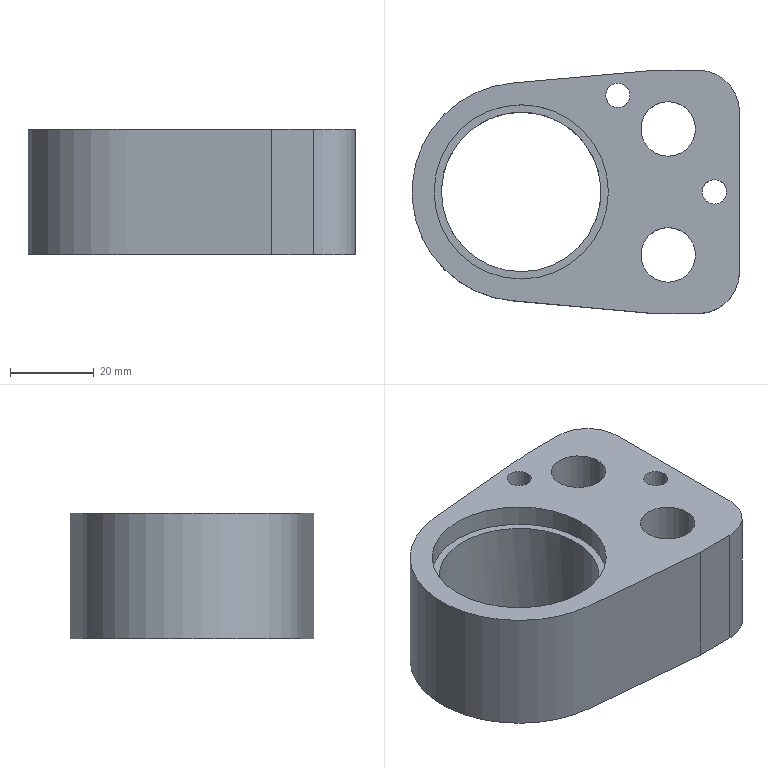Part | NX | features solid 2 | 1 solid | 27 faces | box 78 x 58 x 30 mm | volume 68434 mm3 | plane 14 | cylinder 13 | commonest cylinder face diameters 5.8 x2 8 x2 13 x2 19 x2 20 x2 38 x1
STEP:
#1=CARTESIAN_POINT('',(-809.43,-188.249,101.));
#2=VERTEX_POINT('',#1);
#3=CARTESIAN_POINT('',(-809.43,-188.249,131.));
#4=VERTEX_POINT('',#3);
#5=CARTESIAN_POINT('',(-809.43,-188.249,101.));
#6=DIRECTION('',(0.,0.,1.));
#7=VECTOR('',#6,1000.);
#8=LINE('',#5,#7);
#9=EDGE_CURVE('',#2,#4,#8,.T.);
#10=ORIENTED_EDGE('',*,*,#9,.F.);
#11=CARTESIAN_POINT('',(-809.43,-188.249,101.));
#12=VERTEX_POINT('',#11);
#13=CARTESIAN_POINT('',(-809.43,-214.144,101.));
#14=DIRECTION('',(0.,-1.,0.));
#15=VECTOR('',#14,1000.);
#16=LINE('',#13,#15);
#17=EDGE_CURVE('',#2,#12,#16,.T.);
#18=ORIENTED_EDGE('',*,*,#17,.T.);
#19=CARTESIAN_POINT('',(-809.43,-188.249,131.));
#20=VERTEX_POINT('',#19);
#21=CARTESIAN_POINT('',(-809.43,-188.249,131.));
#22=DIRECTION('',(0.,0.,-1.));
#23=VECTOR('',#22,1000.);
#24=LINE('',#21,#23);
#25=EDGE_CURVE('',#20,#12,#24,.T.);
#26=ORIENTED_EDGE('',*,*,#25,.F.);
#27=CARTESIAN_POINT('',(-809.43,-214.144,131.));
#28=DIRECTION('',(0.,1.,0.));
#29=VECTOR('',#28,1000.);
#30=LINE('',#27,#29);
#31=EDGE_CURVE('',#20,#4,#30,.T.);
#32=ORIENTED_EDGE('',*,*,#31,.T.);
#33=EDGE_LOOP('',(#10,#18,#26,#32));
#34=FACE_BOUND('',#33,.T.);
#35=CARTESIAN_POINT('',(-809.43,-214.144,101.));
#36=DIRECTION('',(-1.,0.,0.));
#37=DIRECTION('',(0.,0.,1.));
#38=AXIS2_PLACEMENT_3D('',#35,#36,#37);
#39=PLANE('',#38);
#40=ADVANCED_FACE('',(#34),#39,.T.);
#41=CARTESIAN_POINT('',(-775.09,-185.144,131.));
#42=VERTEX_POINT('',#41);
#43=CARTESIAN_POINT('',(-795.009,-186.945,131.));
#44=DIRECTION('',(-0.9959,-0.09007,0.));
#45=VECTOR('',#44,1000.);
#46=LINE('',#43,#45);
#47=EDGE_CURVE('',#42,#4,#46,.T.);
#48=ORIENTED_EDGE('',*,*,#47,.T.);
#49=ORIENTED_EDGE('',*,*,#31,.F.);
#50=CARTESIAN_POINT('',(-809.43,-240.038,131.));
#51=VERTEX_POINT('',#50);
#52=CARTESIAN_POINT('',(-807.09,-214.144,131.));
#53=DIRECTION('',(0.,0.,-1.));
#54=DIRECTION('',(0.,-1.,0.));
#55=AXIS2_PLACEMENT_3D('',#52,#53,#54);
#56=CIRCLE('',#55,26.);
#57=EDGE_CURVE('',#51,#20,#56,.T.);
#58=ORIENTED_EDGE('',*,*,#57,.F.);
#59=CARTESIAN_POINT('',(-809.43,-240.038,131.));
#60=VERTEX_POINT('',#59);
#61=CARTESIAN_POINT('',(-809.43,-214.144,131.));
#62=DIRECTION('',(0.,1.,0.));
#63=VECTOR('',#62,1000.);
#64=LINE('',#61,#63);
#65=EDGE_CURVE('',#60,#51,#64,.T.);
#66=ORIENTED_EDGE('',*,*,#65,.F.);
#67=CARTESIAN_POINT('',(-775.09,-243.144,131.));
#68=VERTEX_POINT('',#67);
#69=CARTESIAN_POINT('',(-795.009,-241.342,131.));
#70=DIRECTION('',(0.9959,-0.09007,0.));
#71=VECTOR('',#70,1000.);
#72=LINE('',#69,#71);
#73=EDGE_CURVE('',#60,#68,#72,.T.);
#74=ORIENTED_EDGE('',*,*,#73,.T.);
#75=CARTESIAN_POINT('',(-765.09,-243.144,131.));
#76=VERTEX_POINT('',#75);
#77=CARTESIAN_POINT('',(-792.26,-243.144,131.));
#78=DIRECTION('',(-1.,0.,0.));
#79=VECTOR('',#78,1000.);
#80=LINE('',#77,#79);
#81=EDGE_CURVE('',#76,#68,#80,.T.);
#82=ORIENTED_EDGE('',*,*,#81,.F.);
#83=CARTESIAN_POINT('',(-755.09,-233.144,131.));
#84=VERTEX_POINT('',#83);
#85=CARTESIAN_POINT('',(-765.09,-233.144,131.));
#86=DIRECTION('',(0.,0.,1.));
#87=DIRECTION('',(0.,1.,0.));
#88=AXIS2_PLACEMENT_3D('',#85,#86,#87);
#89=CIRCLE('',#88,10.);
#90=EDGE_CURVE('',#76,#84,#89,.T.);
#91=ORIENTED_EDGE('',*,*,#90,.T.);
#92=CARTESIAN_POINT('',(-755.09,-195.144,131.));
#93=VERTEX_POINT('',#92);
#94=CARTESIAN_POINT('',(-755.09,-214.144,131.));
#95=DIRECTION('',(0.,-1.,0.));
#96=VECTOR('',#95,1000.);
#97=LINE('',#94,#96);
#98=EDGE_CURVE('',#93,#84,#97,.T.);
#99=ORIENTED_EDGE('',*,*,#98,.F.);
#100=CARTESIAN_POINT('',(-765.09,-185.144,131.));
#101=VERTEX_POINT('',#100);
#102=CARTESIAN_POINT('',(-765.09,-195.144,131.));
#103=DIRECTION('',(0.,0.,1.));
#104=DIRECTION('',(0.,1.,0.));
#105=AXIS2_PLACEMENT_3D('',#102,#103,#104);
#106=CIRCLE('',#105,10.);
#107=EDGE_CURVE('',#93,#101,#106,.T.);
#108=ORIENTED_EDGE('',*,*,#107,.T.);
#109=CARTESIAN_POINT('',(-792.26,-185.144,131.));
#110=DIRECTION('',(1.,0.,0.));
#111=VECTOR('',#110,1000.);
#112=LINE('',#109,#111);
#113=EDGE_CURVE('',#42,#101,#112,.T.);
#114=ORIENTED_EDGE('',*,*,#113,.F.);
#115=EDGE_LOOP('',(#48,#49,#58,#66,#74,#82,#91,#99,#108,#114));
#116=FACE_BOUND('',#115,.T.);
#117=CARTESIAN_POINT('',(-761.09,-217.044,131.));
#118=VERTEX_POINT('',#117);
#119=CARTESIAN_POINT('',(-761.09,-214.144,131.));
#120=DIRECTION('',(0.,0.,-1.));
#121=DIRECTION('',(0.,-1.,0.));
#122=AXIS2_PLACEMENT_3D('',#119,#120,#121);
#123=CIRCLE('',#122,2.9);
#124=EDGE_CURVE('',#118,#118,#123,.T.);
#125=ORIENTED_EDGE('',*,*,#124,.T.);
#126=EDGE_LOOP('',(#125));
#127=FACE_BOUND('',#126,.T.);
#128=CARTESIAN_POINT('',(-784.09,-194.044,131.));
#129=VERTEX_POINT('',#128);
#130=CARTESIAN_POINT('',(-784.09,-191.144,131.));
#131=DIRECTION('',(0.,0.,-1.));
#132=DIRECTION('',(0.,-1.,0.));
#133=AXIS2_PLACEMENT_3D('',#130,#131,#132);
#134=CIRCLE('',#133,2.9);
#135=EDGE_CURVE('',#129,#129,#134,.T.);
#136=ORIENTED_EDGE('',*,*,#135,.T.);
#137=EDGE_LOOP('',(#136));
#138=FACE_BOUND('',#137,.T.);
#139=CARTESIAN_POINT('',(-772.09,-205.644,131.));
#140=VERTEX_POINT('',#139);
#141=CARTESIAN_POINT('',(-772.09,-199.144,131.));
#142=DIRECTION('',(0.,0.,-1.));
#143=DIRECTION('',(0.,-1.,0.));
#144=AXIS2_PLACEMENT_3D('',#141,#142,#143);
#145=CIRCLE('',#144,6.5);
#146=EDGE_CURVE('',#140,#140,#145,.T.);
#147=ORIENTED_EDGE('',*,*,#146,.T.);
#148=EDGE_LOOP('',(#147));
#149=FACE_BOUND('',#148,.T.);
#150=CARTESIAN_POINT('',(-772.09,-235.644,131.));
#151=VERTEX_POINT('',#150);
#152=CARTESIAN_POINT('',(-772.09,-229.144,131.));
#153=DIRECTION('',(0.,0.,-1.));
#154=DIRECTION('',(0.,-1.,0.));
#155=AXIS2_PLACEMENT_3D('',#152,#153,#154);
#156=CIRCLE('',#155,6.5);
#157=EDGE_CURVE('',#151,#151,#156,.T.);
#158=ORIENTED_EDGE('',*,*,#157,.T.);
#159=EDGE_LOOP('',(#158));
#160=FACE_BOUND('',#159,.T.);
#161=CARTESIAN_POINT('',(-807.09,-234.894,131.));
#162=VERTEX_POINT('',#161);
#163=CARTESIAN_POINT('',(-807.09,-214.144,131.));
#164=DIRECTION('',(0.,0.,-1.));
#165=DIRECTION('',(0.,-1.,0.));
#166=AXIS2_PLACEMENT_3D('',#163,#164,#165);
#167=CIRCLE('',#166,20.75);
#168=EDGE_CURVE('',#162,#162,#167,.T.);
#169=ORIENTED_EDGE('',*,*,#168,.T.);
#170=EDGE_LOOP('',(#169));
#171=FACE_BOUND('',#170,.T.);
#172=CARTESIAN_POINT('',(-792.26,-214.144,131.));
#173=DIRECTION('',(0.,0.,1.));
#174=DIRECTION('',(0.,1.,0.));
#175=AXIS2_PLACEMENT_3D('',#172,#173,#174);
#176=PLANE('',#175);
#177=ADVANCED_FACE('',(#116,#127,#138,#149,#160,#171),#176,.T.);
#178=CARTESIAN_POINT('',(-775.09,-243.144,101.));
#179=VERTEX_POINT('',#178);
#180=CARTESIAN_POINT('',(-775.09,-243.144,101.));
#181=DIRECTION('',(0.,0.,1.));
#182=VECTOR('',#181,1000.);
#183=LINE('',#180,#182);
#184=EDGE_CURVE('',#179,#68,#183,.T.);
#185=ORIENTED_EDGE('',*,*,#184,.F.);
#186=CARTESIAN_POINT('',(-765.09,-243.144,101.));
#187=VERTEX_POINT('',#186);
#188=CARTESIAN_POINT('',(-792.26,-243.144,101.));
#189=DIRECTION('',(1.,0.,0.));
#190=VECTOR('',#189,1000.);
#191=LINE('',#188,#190);
#192=EDGE_CURVE('',#179,#187,#191,.T.);
#193=ORIENTED_EDGE('',*,*,#192,.T.);
#194=CARTESIAN_POINT('',(-765.09,-243.144,101.));
#195=DIRECTION('',(0.,0.,1.));
#196=VECTOR('',#195,1000.);
#197=LINE('',#194,#196);
#198=EDGE_CURVE('',#187,#76,#197,.T.);
#199=ORIENTED_EDGE('',*,*,#198,.T.);
#200=ORIENTED_EDGE('',*,*,#81,.T.);
#201=EDGE_LOOP('',(#185,#193,#199,#200));
#202=FACE_BOUND('',#201,.T.);
#203=CARTESIAN_POINT('',(-792.26,-243.144,101.));
#204=DIRECTION('',(0.,-1.,0.));
#205=DIRECTION('',(0.,0.,1.));
#206=AXIS2_PLACEMENT_3D('',#203,#204,#205);
#207=PLANE('',#206);
#208=ADVANCED_FACE('',(#202),#207,.T.);
#209=CARTESIAN_POINT('',(-809.43,-240.038,101.));
#210=VERTEX_POINT('',#209);
#211=CARTESIAN_POINT('',(-809.43,-240.038,101.));
#212=DIRECTION('',(0.,0.,-1.));
#213=VECTOR('',#212,1000.);
#214=LINE('',#211,#213);
#215=EDGE_CURVE('',#60,#210,#214,.T.);
#216=ORIENTED_EDGE('',*,*,#215,.F.);
#217=ORIENTED_EDGE('',*,*,#65,.T.);
#218=CARTESIAN_POINT('',(-809.43,-240.038,101.));
#219=VERTEX_POINT('',#218);
#220=CARTESIAN_POINT('',(-809.43,-240.038,131.));
#221=DIRECTION('',(0.,0.,-1.));
#222=VECTOR('',#221,1000.);
#223=LINE('',#220,#222);
#224=EDGE_CURVE('',#219,#51,#223,.F.);
#225=ORIENTED_EDGE('',*,*,#224,.F.);
#226=CARTESIAN_POINT('',(-809.43,-214.144,101.));
#227=DIRECTION('',(0.,-1.,0.));
#228=VECTOR('',#227,1000.);
#229=LINE('',#226,#228);
#230=EDGE_CURVE('',#219,#210,#229,.T.);
#231=ORIENTED_EDGE('',*,*,#230,.T.);
#232=EDGE_LOOP('',(#216,#217,#225,#231));
#233=FACE_BOUND('',#232,.T.);
#234=CARTESIAN_POINT('',(-809.43,-214.144,101.));
#235=DIRECTION('',(-1.,0.,0.));
#236=DIRECTION('',(0.,0.,1.));
#237=AXIS2_PLACEMENT_3D('',#234,#235,#236);
#238=PLANE('',#237);
#239=ADVANCED_FACE('',(#233),#238,.T.);
#240=CARTESIAN_POINT('',(-775.09,-185.144,101.));
#241=VERTEX_POINT('',#240);
#242=CARTESIAN_POINT('',(-795.009,-186.945,101.));
#243=DIRECTION('',(0.9959,0.09007,0.));
#244=VECTOR('',#243,1000.);
#245=LINE('',#242,#244);
#246=EDGE_CURVE('',#2,#241,#245,.T.);
#247=ORIENTED_EDGE('',*,*,#246,.T.);
#248=CARTESIAN_POINT('',(-765.09,-185.144,101.));
#249=VERTEX_POINT('',#248);
#250=CARTESIAN_POINT('',(-792.26,-185.144,101.));
#251=DIRECTION('',(-1.,0.,0.));
#252=VECTOR('',#251,1000.);
#253=LINE('',#250,#252);
#254=EDGE_CURVE('',#249,#241,#253,.T.);
#255=ORIENTED_EDGE('',*,*,#254,.F.);
#256=CARTESIAN_POINT('',(-755.09,-195.144,101.));
#257=VERTEX_POINT('',#256);
#258=CARTESIAN_POINT('',(-765.09,-195.144,101.));
#259=DIRECTION('',(0.,0.,-1.));
#260=DIRECTION('',(0.,-1.,0.));
#261=AXIS2_PLACEMENT_3D('',#258,#259,#260);
#262=CIRCLE('',#261,10.);
#263=EDGE_CURVE('',#249,#257,#262,.T.);
#264=ORIENTED_EDGE('',*,*,#263,.T.);
#265=CARTESIAN_POINT('',(-755.09,-233.144,101.));
#266=VERTEX_POINT('',#265);
#267=CARTESIAN_POINT('',(-755.09,-214.144,101.));
#268=DIRECTION('',(0.,1.,0.));
#269=VECTOR('',#268,1000.);
#270=LINE('',#267,#269);
#271=EDGE_CURVE('',#266,#257,#270,.T.);
#272=ORIENTED_EDGE('',*,*,#271,.F.);
#273=CARTESIAN_POINT('',(-765.09,-233.144,101.));
#274=DIRECTION('',(0.,0.,-1.));
#275=DIRECTION('',(0.,-1.,0.));
#276=AXIS2_PLACEMENT_3D('',#273,#274,#275);
#277=CIRCLE('',#276,10.);
#278=EDGE_CURVE('',#266,#187,#277,.T.);
#279=ORIENTED_EDGE('',*,*,#278,.T.);
#280=ORIENTED_EDGE('',*,*,#192,.F.);
#281=CARTESIAN_POINT('',(-795.009,-241.342,101.));
#282=DIRECTION('',(-0.9959,0.09007,0.));
#283=VECTOR('',#282,1000.);
#284=LINE('',#281,#283);
#285=EDGE_CURVE('',#179,#210,#284,.T.);
#286=ORIENTED_EDGE('',*,*,#285,.T.);
#287=ORIENTED_EDGE('',*,*,#230,.F.);
#288=CARTESIAN_POINT('',(-807.09,-214.144,101.));
#289=DIRECTION('',(0.,0.,1.));
#290=DIRECTION('',(0.,1.,0.));
#291=AXIS2_PLACEMENT_3D('',#288,#289,#290);
#292=CIRCLE('',#291,26.);
#293=EDGE_CURVE('',#12,#219,#292,.T.);
#294=ORIENTED_EDGE('',*,*,#293,.F.);
#295=ORIENTED_EDGE('',*,*,#17,.F.);
#296=EDGE_LOOP('',(#247,#255,#264,#272,#279,#280,#286,#287,#294,#295));
#297=FACE_BOUND('',#296,.T.);
#298=CARTESIAN_POINT('',(-761.09,-210.144,101.));
#299=VERTEX_POINT('',#298);
#300=CARTESIAN_POINT('',(-761.09,-214.144,101.));
#301=DIRECTION('',(0.,0.,1.));
#302=DIRECTION('',(0.,1.,0.));
#303=AXIS2_PLACEMENT_3D('',#300,#301,#302);
#304=CIRCLE('',#303,4.);
#305=EDGE_CURVE('',#299,#299,#304,.T.);
#306=ORIENTED_EDGE('',*,*,#305,.T.);
#307=EDGE_LOOP('',(#306));
#308=FACE_BOUND('',#307,.T.);
#309=CARTESIAN_POINT('',(-784.09,-187.144,101.));
#310=VERTEX_POINT('',#309);
#311=CARTESIAN_POINT('',(-784.09,-191.144,101.));
#312=DIRECTION('',(0.,0.,1.));
#313=DIRECTION('',(0.,1.,0.));
#314=AXIS2_PLACEMENT_3D('',#311,#312,#313);
#315=CIRCLE('',#314,4.);
#316=EDGE_CURVE('',#310,#310,#315,.T.);
#317=ORIENTED_EDGE('',*,*,#316,.T.);
#318=EDGE_LOOP('',(#317));
#319=FACE_BOUND('',#318,.T.);
#320=CARTESIAN_POINT('',(-772.09,-189.644,101.));
#321=VERTEX_POINT('',#320);
#322=CARTESIAN_POINT('',(-772.09,-199.144,101.));
#323=DIRECTION('',(0.,0.,1.));
#324=DIRECTION('',(0.,1.,0.));
#325=AXIS2_PLACEMENT_3D('',#322,#323,#324);
#326=CIRCLE('',#325,9.5);
#327=EDGE_CURVE('',#321,#321,#326,.T.);
#328=ORIENTED_EDGE('',*,*,#327,.T.);
#329=EDGE_LOOP('',(#328));
#330=FACE_BOUND('',#329,.T.);
#331=CARTESIAN_POINT('',(-772.09,-219.644,101.));
#332=VERTEX_POINT('',#331);
#333=CARTESIAN_POINT('',(-772.09,-229.144,101.));
#334=DIRECTION('',(0.,0.,1.));
#335=DIRECTION('',(0.,1.,0.));
#336=AXIS2_PLACEMENT_3D('',#333,#334,#335);
#337=CIRCLE('',#336,9.5);
#338=EDGE_CURVE('',#332,#332,#337,.T.);
#339=ORIENTED_EDGE('',*,*,#338,.T.);
#340=EDGE_LOOP('',(#339));
#341=FACE_BOUND('',#340,.T.);
#342=CARTESIAN_POINT('',(-807.09,-195.144,101.));
#343=VERTEX_POINT('',#342);
#344=CARTESIAN_POINT('',(-807.09,-214.144,101.));
#345=DIRECTION('',(0.,0.,1.));
#346=DIRECTION('',(0.,1.,0.));
#347=AXIS2_PLACEMENT_3D('',#344,#345,#346);
#348=CIRCLE('',#347,19.);
#349=EDGE_CURVE('',#343,#343,#348,.T.);
#350=ORIENTED_EDGE('',*,*,#349,.T.);
#351=EDGE_LOOP('',(#350));
#352=FACE_BOUND('',#351,.T.);
#353=CARTESIAN_POINT('',(-792.26,-214.144,101.));
#354=DIRECTION('',(0.,0.,-1.));
#355=DIRECTION('',(0.,-1.,0.));
#356=AXIS2_PLACEMENT_3D('',#353,#354,#355);
#357=PLANE('',#356);
#358=ADVANCED_FACE('',(#297,#308,#319,#330,#341,#352),#357,.T.);
#359=CARTESIAN_POINT('',(-775.09,-185.144,101.));
#360=DIRECTION('',(0.,0.,1.));
#361=VECTOR('',#360,1000.);
#362=LINE('',#359,#361);
#363=EDGE_CURVE('',#241,#42,#362,.T.);
#364=ORIENTED_EDGE('',*,*,#363,.T.);
#365=ORIENTED_EDGE('',*,*,#113,.T.);
#366=CARTESIAN_POINT('',(-765.09,-185.144,101.));
#367=DIRECTION('',(0.,0.,1.));
#368=VECTOR('',#367,1000.);
#369=LINE('',#366,#368);
#370=EDGE_CURVE('',#101,#249,#369,.F.);
#371=ORIENTED_EDGE('',*,*,#370,.T.);
#372=ORIENTED_EDGE('',*,*,#254,.T.);
#373=EDGE_LOOP('',(#364,#365,#371,#372));
#374=FACE_BOUND('',#373,.T.);
#375=CARTESIAN_POINT('',(-792.26,-185.144,101.));
#376=DIRECTION('',(0.,1.,0.));
#377=DIRECTION('',(0.,0.,-1.));
#378=AXIS2_PLACEMENT_3D('',#375,#376,#377);
#379=PLANE('',#378);
#380=ADVANCED_FACE('',(#374),#379,.T.);
#381=ORIENTED_EDGE('',*,*,#57,.T.);
#382=ORIENTED_EDGE('',*,*,#25,.T.);
#383=ORIENTED_EDGE('',*,*,#293,.T.);
#384=ORIENTED_EDGE('',*,*,#224,.T.);
#385=EDGE_LOOP('',(#381,#382,#383,#384));
#386=FACE_BOUND('',#385,.T.);
#387=CARTESIAN_POINT('',(-807.09,-214.144,131.));
#388=DIRECTION('',(0.,0.,-1.));
#389=DIRECTION('',(0.,-1.,0.));
#390=AXIS2_PLACEMENT_3D('',#387,#388,#389);
#391=CYLINDRICAL_SURFACE('',#390,26.);
#392=ADVANCED_FACE('',(#386),#391,.T.);
#393=ORIENTED_EDGE('',*,*,#271,.T.);
#394=CARTESIAN_POINT('',(-755.09,-195.144,101.));
#395=DIRECTION('',(0.,0.,1.));
#396=VECTOR('',#395,1000.);
#397=LINE('',#394,#396);
#398=EDGE_CURVE('',#257,#93,#397,.T.);
#399=ORIENTED_EDGE('',*,*,#398,.T.);
#400=ORIENTED_EDGE('',*,*,#98,.T.);
#401=CARTESIAN_POINT('',(-755.09,-233.144,101.));
#402=DIRECTION('',(0.,0.,1.));
#403=VECTOR('',#402,1000.);
#404=LINE('',#401,#403);
#405=EDGE_CURVE('',#84,#266,#404,.F.);
#406=ORIENTED_EDGE('',*,*,#405,.T.);
#407=EDGE_LOOP('',(#393,#399,#400,#406));
#408=FACE_BOUND('',#407,.T.);
#409=CARTESIAN_POINT('',(-755.09,-214.144,101.));
#410=DIRECTION('',(1.,0.,0.));
#411=DIRECTION('',(0.,0.,-1.));
#412=AXIS2_PLACEMENT_3D('',#409,#410,#411);
#413=PLANE('',#412);
#414=ADVANCED_FACE('',(#408),#413,.T.);
#415=CARTESIAN_POINT('',(-807.09,-233.144,126.));
#416=VERTEX_POINT('',#415);
#417=CARTESIAN_POINT('',(-807.09,-214.144,126.));
#418=DIRECTION('',(0.,0.,-1.));
#419=DIRECTION('',(0.,-1.,0.));
#420=AXIS2_PLACEMENT_3D('',#417,#418,#419);
#421=CIRCLE('',#420,19.);
#422=EDGE_CURVE('',#416,#416,#421,.T.);
#423=ORIENTED_EDGE('',*,*,#422,.T.);
#424=EDGE_LOOP('',(#423));
#425=FACE_BOUND('',#424,.T.);
#426=CARTESIAN_POINT('',(-807.09,-193.394,126.));
#427=VERTEX_POINT('',#426);
#428=CARTESIAN_POINT('',(-807.09,-214.144,126.));
#429=DIRECTION('',(0.,0.,1.));
#430=DIRECTION('',(0.,1.,0.));
#431=AXIS2_PLACEMENT_3D('',#428,#429,#430);
#432=CIRCLE('',#431,20.75);
#433=EDGE_CURVE('',#427,#427,#432,.T.);
#434=ORIENTED_EDGE('',*,*,#433,.T.);
#435=EDGE_LOOP('',(#434));
#436=FACE_BOUND('',#435,.T.);
#437=CARTESIAN_POINT('',(-807.09,-214.144,126.));
#438=DIRECTION('',(0.,0.,-1.));
#439=DIRECTION('',(0.,-1.,0.));
#440=AXIS2_PLACEMENT_3D('',#437,#438,#439);
#441=PLANE('',#440);
#442=ADVANCED_FACE('',(#425,#436),#441,.F.);
#443=ORIENTED_EDGE('',*,*,#433,.F.);
#444=EDGE_LOOP('',(#443));
#445=FACE_BOUND('',#444,.T.);
#446=ORIENTED_EDGE('',*,*,#168,.F.);
#447=EDGE_LOOP('',(#446));
#448=FACE_BOUND('',#447,.T.);
#449=CARTESIAN_POINT('',(-807.09,-214.144,131.));
#450=DIRECTION('',(0.,0.,-1.));
#451=DIRECTION('',(0.,-1.,0.));
#452=AXIS2_PLACEMENT_3D('',#449,#450,#451);
#453=CYLINDRICAL_SURFACE('',#452,20.75);
#454=ADVANCED_FACE('',(#445,#448),#453,.F.);
#455=ORIENTED_EDGE('',*,*,#349,.F.);
#456=EDGE_LOOP('',(#455));
#457=FACE_BOUND('',#456,.T.);
#458=ORIENTED_EDGE('',*,*,#422,.F.);
#459=EDGE_LOOP('',(#458));
#460=FACE_BOUND('',#459,.T.);
#461=CARTESIAN_POINT('',(-807.09,-214.144,126.));
#462=DIRECTION('',(0.,0.,-1.));
#463=DIRECTION('',(0.,-1.,0.));
#464=AXIS2_PLACEMENT_3D('',#461,#462,#463);
#465=CYLINDRICAL_SURFACE('',#464,19.);
#466=ADVANCED_FACE('',(#457,#460),#465,.F.);
#467=CARTESIAN_POINT('',(-772.09,-222.644,115.));
#468=VERTEX_POINT('',#467);
#469=CARTESIAN_POINT('',(-772.09,-229.144,115.));
#470=DIRECTION('',(0.,0.,1.));
#471=DIRECTION('',(0.,1.,0.));
#472=AXIS2_PLACEMENT_3D('',#469,#470,#471);
#473=CIRCLE('',#472,6.5);
#474=EDGE_CURVE('',#468,#468,#473,.F.);
#475=ORIENTED_EDGE('',*,*,#474,.T.);
#476=EDGE_LOOP('',(#475));
#477=FACE_BOUND('',#476,.T.);
#478=ORIENTED_EDGE('',*,*,#157,.F.);
#479=EDGE_LOOP('',(#478));
#480=FACE_BOUND('',#479,.T.);
#481=CARTESIAN_POINT('',(-772.09,-229.144,131.));
#482=DIRECTION('',(0.,0.,-1.));
#483=DIRECTION('',(0.,-1.,0.));
#484=AXIS2_PLACEMENT_3D('',#481,#482,#483);
#485=CYLINDRICAL_SURFACE('',#484,6.5);
#486=ADVANCED_FACE('',(#477,#480),#485,.F.);
#487=CARTESIAN_POINT('',(-772.09,-238.644,115.));
#488=VERTEX_POINT('',#487);
#489=CARTESIAN_POINT('',(-772.09,-229.144,115.));
#490=DIRECTION('',(0.,0.,-1.));
#491=DIRECTION('',(0.,-1.,0.));
#492=AXIS2_PLACEMENT_3D('',#489,#490,#491);
#493=CIRCLE('',#492,9.5);
#494=EDGE_CURVE('',#488,#488,#493,.T.);
#495=ORIENTED_EDGE('',*,*,#494,.T.);
#496=EDGE_LOOP('',(#495));
#497=FACE_BOUND('',#496,.T.);
#498=ORIENTED_EDGE('',*,*,#474,.F.);
#499=EDGE_LOOP('',(#498));
#500=FACE_BOUND('',#499,.T.);
#501=CARTESIAN_POINT('',(-772.09,-229.144,115.));
#502=DIRECTION('',(0.,0.,1.));
#503=DIRECTION('',(0.,1.,0.));
#504=AXIS2_PLACEMENT_3D('',#501,#502,#503);
#505=PLANE('',#504);
#506=ADVANCED_FACE('',(#497,#500),#505,.F.);
#507=ORIENTED_EDGE('',*,*,#338,.F.);
#508=EDGE_LOOP('',(#507));
#509=FACE_BOUND('',#508,.T.);
#510=ORIENTED_EDGE('',*,*,#494,.F.);
#511=EDGE_LOOP('',(#510));
#512=FACE_BOUND('',#511,.T.);
#513=CARTESIAN_POINT('',(-772.09,-229.144,115.));
#514=DIRECTION('',(0.,0.,-1.));
#515=DIRECTION('',(0.,-1.,0.));
#516=AXIS2_PLACEMENT_3D('',#513,#514,#515);
#517=CYLINDRICAL_SURFACE('',#516,9.5);
#518=ADVANCED_FACE('',(#509,#512),#517,.F.);
#519=CARTESIAN_POINT('',(-772.09,-192.644,115.));
#520=VERTEX_POINT('',#519);
#521=CARTESIAN_POINT('',(-772.09,-199.144,115.));
#522=DIRECTION('',(0.,0.,1.));
#523=DIRECTION('',(0.,1.,0.));
#524=AXIS2_PLACEMENT_3D('',#521,#522,#523);
#525=CIRCLE('',#524,6.5);
#526=EDGE_CURVE('',#520,#520,#525,.F.);
#527=ORIENTED_EDGE('',*,*,#526,.T.);
#528=EDGE_LOOP('',(#527));
#529=FACE_BOUND('',#528,.T.);
#530=ORIENTED_EDGE('',*,*,#146,.F.);
#531=EDGE_LOOP('',(#530));
#532=FACE_BOUND('',#531,.T.);
#533=CARTESIAN_POINT('',(-772.09,-199.144,131.));
#534=DIRECTION('',(0.,0.,-1.));
#535=DIRECTION('',(0.,-1.,0.));
#536=AXIS2_PLACEMENT_3D('',#533,#534,#535);
#537=CYLINDRICAL_SURFACE('',#536,6.5);
#538=ADVANCED_FACE('',(#529,#532),#537,.F.);
#539=CARTESIAN_POINT('',(-772.09,-208.644,115.));
#540=VERTEX_POINT('',#539);
#541=CARTESIAN_POINT('',(-772.09,-199.144,115.));
#542=DIRECTION('',(0.,0.,-1.));
#543=DIRECTION('',(0.,-1.,0.));
#544=AXIS2_PLACEMENT_3D('',#541,#542,#543);
#545=CIRCLE('',#544,9.5);
#546=EDGE_CURVE('',#540,#540,#545,.T.);
#547=ORIENTED_EDGE('',*,*,#546,.T.);
#548=EDGE_LOOP('',(#547));
#549=FACE_BOUND('',#548,.T.);
#550=ORIENTED_EDGE('',*,*,#526,.F.);
#551=EDGE_LOOP('',(#550));
#552=FACE_BOUND('',#551,.T.);
#553=CARTESIAN_POINT('',(-772.09,-199.144,115.));
#554=DIRECTION('',(0.,0.,1.));
#555=DIRECTION('',(0.,1.,0.));
#556=AXIS2_PLACEMENT_3D('',#553,#554,#555);
#557=PLANE('',#556);
#558=ADVANCED_FACE('',(#549,#552),#557,.F.);
#559=ORIENTED_EDGE('',*,*,#327,.F.);
#560=EDGE_LOOP('',(#559));
#561=FACE_BOUND('',#560,.T.);
#562=ORIENTED_EDGE('',*,*,#546,.F.);
#563=EDGE_LOOP('',(#562));
#564=FACE_BOUND('',#563,.T.);
#565=CARTESIAN_POINT('',(-772.09,-199.144,115.));
#566=DIRECTION('',(0.,0.,-1.));
#567=DIRECTION('',(0.,-1.,0.));
#568=AXIS2_PLACEMENT_3D('',#565,#566,#567);
#569=CYLINDRICAL_SURFACE('',#568,9.5);
#570=ADVANCED_FACE('',(#561,#564),#569,.F.);
#571=CARTESIAN_POINT('',(-784.09,-188.244,121.));
#572=VERTEX_POINT('',#571);
#573=CARTESIAN_POINT('',(-784.09,-191.144,121.));
#574=DIRECTION('',(0.,0.,1.));
#575=DIRECTION('',(0.,1.,0.));
#576=AXIS2_PLACEMENT_3D('',#573,#574,#575);
#577=CIRCLE('',#576,2.9);
#578=EDGE_CURVE('',#572,#572,#577,.F.);
#579=ORIENTED_EDGE('',*,*,#578,.T.);
#580=EDGE_LOOP('',(#579));
#581=FACE_BOUND('',#580,.T.);
#582=ORIENTED_EDGE('',*,*,#135,.F.);
#583=EDGE_LOOP('',(#582));
#584=FACE_BOUND('',#583,.T.);
#585=CARTESIAN_POINT('',(-784.09,-191.144,131.));
#586=DIRECTION('',(0.,0.,-1.));
#587=DIRECTION('',(0.,-1.,0.));
#588=AXIS2_PLACEMENT_3D('',#585,#586,#587);
#589=CYLINDRICAL_SURFACE('',#588,2.9);
#590=ADVANCED_FACE('',(#581,#584),#589,.F.);
#591=CARTESIAN_POINT('',(-784.09,-195.144,121.));
#592=VERTEX_POINT('',#591);
#593=CARTESIAN_POINT('',(-784.09,-191.144,121.));
#594=DIRECTION('',(0.,0.,-1.));
#595=DIRECTION('',(0.,-1.,0.));
#596=AXIS2_PLACEMENT_3D('',#593,#594,#595);
#597=CIRCLE('',#596,4.);
#598=EDGE_CURVE('',#592,#592,#597,.T.);
#599=ORIENTED_EDGE('',*,*,#598,.T.);
#600=EDGE_LOOP('',(#599));
#601=FACE_BOUND('',#600,.T.);
#602=ORIENTED_EDGE('',*,*,#578,.F.);
#603=EDGE_LOOP('',(#602));
#604=FACE_BOUND('',#603,.T.);
#605=CARTESIAN_POINT('',(-784.09,-191.144,121.));
#606=DIRECTION('',(0.,0.,1.));
#607=DIRECTION('',(0.,1.,0.));
#608=AXIS2_PLACEMENT_3D('',#605,#606,#607);
#609=PLANE('',#608);
#610=ADVANCED_FACE('',(#601,#604),#609,.F.);
#611=ORIENTED_EDGE('',*,*,#316,.F.);
#612=EDGE_LOOP('',(#611));
#613=FACE_BOUND('',#612,.T.);
#614=ORIENTED_EDGE('',*,*,#598,.F.);
#615=EDGE_LOOP('',(#614));
#616=FACE_BOUND('',#615,.T.);
#617=CARTESIAN_POINT('',(-784.09,-191.144,121.));
#618=DIRECTION('',(0.,0.,-1.));
#619=DIRECTION('',(0.,-1.,0.));
#620=AXIS2_PLACEMENT_3D('',#617,#618,#619);
#621=CYLINDRICAL_SURFACE('',#620,4.);
#622=ADVANCED_FACE('',(#613,#616),#621,.F.);
#623=CARTESIAN_POINT('',(-761.09,-211.244,121.));
#624=VERTEX_POINT('',#623);
#625=CARTESIAN_POINT('',(-761.09,-214.144,121.));
#626=DIRECTION('',(0.,0.,1.));
#627=DIRECTION('',(0.,1.,0.));
#628=AXIS2_PLACEMENT_3D('',#625,#626,#627);
#629=CIRCLE('',#628,2.9);
#630=EDGE_CURVE('',#624,#624,#629,.F.);
#631=ORIENTED_EDGE('',*,*,#630,.T.);
#632=EDGE_LOOP('',(#631));
#633=FACE_BOUND('',#632,.T.);
#634=ORIENTED_EDGE('',*,*,#124,.F.);
#635=EDGE_LOOP('',(#634));
#636=FACE_BOUND('',#635,.T.);
#637=CARTESIAN_POINT('',(-761.09,-214.144,131.));
#638=DIRECTION('',(0.,0.,-1.));
#639=DIRECTION('',(0.,-1.,0.));
#640=AXIS2_PLACEMENT_3D('',#637,#638,#639);
#641=CYLINDRICAL_SURFACE('',#640,2.9);
#642=ADVANCED_FACE('',(#633,#636),#641,.F.);
#643=CARTESIAN_POINT('',(-761.09,-218.144,121.));
#644=VERTEX_POINT('',#643);
#645=CARTESIAN_POINT('',(-761.09,-214.144,121.));
#646=DIRECTION('',(0.,0.,-1.));
#647=DIRECTION('',(0.,-1.,0.));
#648=AXIS2_PLACEMENT_3D('',#645,#646,#647);
#649=CIRCLE('',#648,4.);
#650=EDGE_CURVE('',#644,#644,#649,.T.);
#651=ORIENTED_EDGE('',*,*,#650,.T.);
#652=EDGE_LOOP('',(#651));
#653=FACE_BOUND('',#652,.T.);
#654=ORIENTED_EDGE('',*,*,#630,.F.);
#655=EDGE_LOOP('',(#654));
#656=FACE_BOUND('',#655,.T.);
#657=CARTESIAN_POINT('',(-761.09,-214.144,121.));
#658=DIRECTION('',(0.,0.,1.));
#659=DIRECTION('',(0.,1.,0.));
#660=AXIS2_PLACEMENT_3D('',#657,#658,#659);
#661=PLANE('',#660);
#662=ADVANCED_FACE('',(#653,#656),#661,.F.);
#663=ORIENTED_EDGE('',*,*,#305,.F.);
#664=EDGE_LOOP('',(#663));
#665=FACE_BOUND('',#664,.T.);
#666=ORIENTED_EDGE('',*,*,#650,.F.);
#667=EDGE_LOOP('',(#666));
#668=FACE_BOUND('',#667,.T.);
#669=CARTESIAN_POINT('',(-761.09,-214.144,121.));
#670=DIRECTION('',(0.,0.,-1.));
#671=DIRECTION('',(0.,-1.,0.));
#672=AXIS2_PLACEMENT_3D('',#669,#670,#671);
#673=CYLINDRICAL_SURFACE('',#672,4.);
#674=ADVANCED_FACE('',(#665,#668),#673,.F.);
#675=ORIENTED_EDGE('',*,*,#263,.F.);
#676=ORIENTED_EDGE('',*,*,#370,.F.);
#677=ORIENTED_EDGE('',*,*,#107,.F.);
#678=ORIENTED_EDGE('',*,*,#398,.F.);
#679=EDGE_LOOP('',(#675,#676,#677,#678));
#680=FACE_BOUND('',#679,.T.);
#681=CARTESIAN_POINT('',(-765.09,-195.144,101.));
#682=DIRECTION('',(0.,0.,1.));
#683=DIRECTION('',(0.,1.,0.));
#684=AXIS2_PLACEMENT_3D('',#681,#682,#683);
#685=CYLINDRICAL_SURFACE('',#684,10.);
#686=ADVANCED_FACE('',(#680),#685,.T.);
#687=ORIENTED_EDGE('',*,*,#278,.F.);
#688=ORIENTED_EDGE('',*,*,#405,.F.);
#689=ORIENTED_EDGE('',*,*,#90,.F.);
#690=ORIENTED_EDGE('',*,*,#198,.F.);
#691=EDGE_LOOP('',(#687,#688,#689,#690));
#692=FACE_BOUND('',#691,.T.);
#693=CARTESIAN_POINT('',(-765.09,-233.144,101.));
#694=DIRECTION('',(0.,0.,1.));
#695=DIRECTION('',(0.,1.,0.));
#696=AXIS2_PLACEMENT_3D('',#693,#694,#695);
#697=CYLINDRICAL_SURFACE('',#696,10.);
#698=ADVANCED_FACE('',(#692),#697,.T.);
#699=ORIENTED_EDGE('',*,*,#215,.T.);
#700=ORIENTED_EDGE('',*,*,#285,.F.);
#701=ORIENTED_EDGE('',*,*,#184,.T.);
#702=ORIENTED_EDGE('',*,*,#73,.F.);
#703=EDGE_LOOP('',(#699,#700,#701,#702));
#704=FACE_BOUND('',#703,.T.);
#705=CARTESIAN_POINT('',(-795.009,-241.342,101.));
#706=DIRECTION('',(0.09007,0.9959,0.));
#707=DIRECTION('',(0.,0.,-1.));
#708=AXIS2_PLACEMENT_3D('',#705,#706,#707);
#709=PLANE('',#708);
#710=ADVANCED_FACE('',(#704),#709,.F.);
#711=ORIENTED_EDGE('',*,*,#9,.T.);
#712=ORIENTED_EDGE('',*,*,#47,.F.);
#713=ORIENTED_EDGE('',*,*,#363,.F.);
#714=ORIENTED_EDGE('',*,*,#246,.F.);
#715=EDGE_LOOP('',(#711,#712,#713,#714));
#716=FACE_BOUND('',#715,.T.);
#717=CARTESIAN_POINT('',(-795.009,-186.945,101.));
#718=DIRECTION('',(0.09007,-0.9959,0.));
#719=DIRECTION('',(0.,0.,1.));
#720=AXIS2_PLACEMENT_3D('',#717,#718,#719);
#721=PLANE('',#720);
#722=ADVANCED_FACE('',(#716),#721,.F.);
#723=CLOSED_SHELL('',(#40,#177,#208,#239,#358,#380,#392,#414,#442,#454,#466,#486,#506,#518,#538,#558,#570,#590,#610,#622,#642,#662,#674,#686,#698,#710,#722));
#724=MANIFOLD_SOLID_BREP('',#723);
#725=(LENGTH_UNIT()NAMED_UNIT(*)SI_UNIT(.MILLI.,.METRE.));
#726=UNCERTAINTY_MEASURE_WITH_UNIT(LENGTH_MEASURE(0.00001),#725,'','');
#727=(NAMED_UNIT(*)PLANE_ANGLE_UNIT()SI_UNIT($,.RADIAN.));
#728=(NAMED_UNIT(*)SI_UNIT($,.STERADIAN.)SOLID_ANGLE_UNIT());
#729=(GEOMETRIC_REPRESENTATION_CONTEXT(3)GLOBAL_UNCERTAINTY_ASSIGNED_CONTEXT((#726))GLOBAL_UNIT_ASSIGNED_CONTEXT((#725,#727,#728))REPRESENTATION_CONTEXT('',''));
#730=ADVANCED_BREP_SHAPE_REPRESENTATION('',(#724),#729);